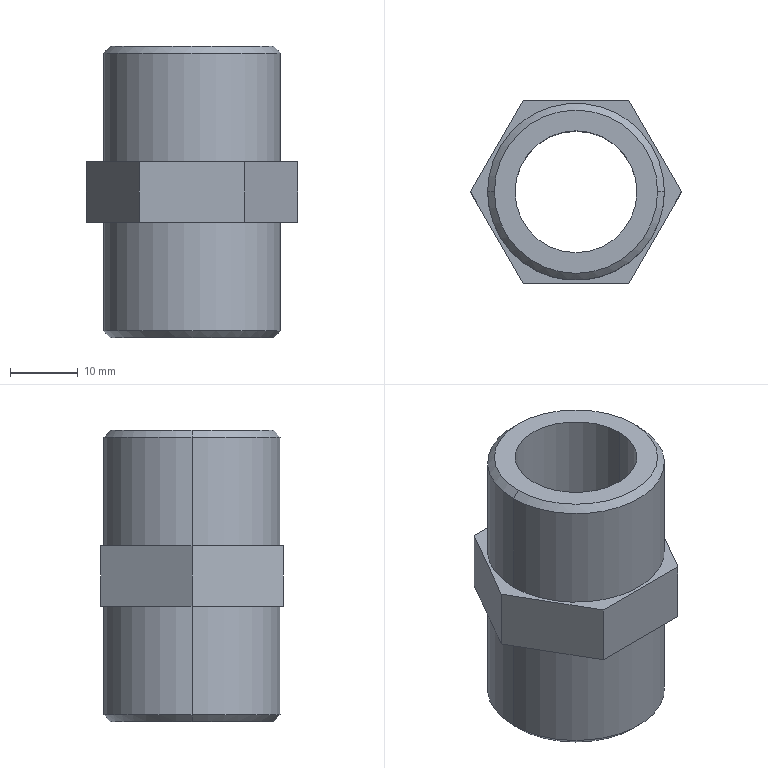Part | SolidWorks | features ICE 2, Chamfer 1, Extrusion 1, MirrorPattern 1 | 1 solid | 20 faces | box 31.177 x 27 x 43 mm | volume 12851 mm3 | plane 10 | cylinder 6 | cone 4 | commonest cylinder face diameters 26.1 x4 18 x2
STEP:
#1=CARTESIAN_POINT('',(12.05,0.,21.5));
#2=VERTEX_POINT('',#1);
#3=CARTESIAN_POINT('',(-12.05,0.,21.5));
#4=VERTEX_POINT('',#3);
#5=CARTESIAN_POINT('',(0.,0.,21.5));
#6=DIRECTION('',(0.,0.,1.));
#7=DIRECTION('',(1.,0.,0.));
#8=AXIS2_PLACEMENT_3D('',#5,#6,#7);
#9=CIRCLE('',#8,12.05);
#10=EDGE_CURVE('',#2,#4,#9,.T.);
#11=ORIENTED_EDGE('',*,*,#10,.F.);
#12=CARTESIAN_POINT('',(13.05,0.,20.5));
#13=VERTEX_POINT('',#12);
#14=CARTESIAN_POINT('',(13.05,0.,20.5));
#15=DIRECTION('',(0.7071,0.,-0.7071));
#16=VECTOR('',#15,1000.);
#17=LINE('',#14,#16);
#18=EDGE_CURVE('',#2,#13,#17,.T.);
#19=ORIENTED_EDGE('',*,*,#18,.T.);
#20=CARTESIAN_POINT('',(-13.05,0.,20.5));
#21=VERTEX_POINT('',#20);
#22=CARTESIAN_POINT('',(0.,0.,20.5));
#23=DIRECTION('',(0.,0.,-1.));
#24=DIRECTION('',(1.,0.,0.));
#25=AXIS2_PLACEMENT_3D('',#22,#23,#24);
#26=CIRCLE('',#25,13.05);
#27=EDGE_CURVE('',#21,#13,#26,.T.);
#28=ORIENTED_EDGE('',*,*,#27,.F.);
#29=CARTESIAN_POINT('',(-13.05,0.,20.5));
#30=DIRECTION('',(-0.7071,0.,-0.7071));
#31=VECTOR('',#30,1000.);
#32=LINE('',#29,#31);
#33=EDGE_CURVE('',#4,#21,#32,.T.);
#34=ORIENTED_EDGE('',*,*,#33,.F.);
#35=EDGE_LOOP('',(#11,#19,#28,#34));
#36=FACE_OUTER_BOUND('',#35,.T.);
#37=CARTESIAN_POINT('',(0.,0.,20.5));
#38=DIRECTION('',(0.,0.,-1.));
#39=DIRECTION('',(-1.,0.,0.));
#40=AXIS2_PLACEMENT_3D('',#37,#38,#39);
#41=CONICAL_SURFACE('',#40,13.05,0.7854);
#42=ADVANCED_FACE('',(#36),#41,.T.);
#43=CARTESIAN_POINT('',(-12.05,0.,-21.5));
#44=VERTEX_POINT('',#43);
#45=CARTESIAN_POINT('',(12.05,0.,-21.5));
#46=VERTEX_POINT('',#45);
#47=CARTESIAN_POINT('',(0.,0.,-21.5));
#48=DIRECTION('',(0.,0.,-1.));
#49=DIRECTION('',(-1.,0.,0.));
#50=AXIS2_PLACEMENT_3D('',#47,#48,#49);
#51=CIRCLE('',#50,12.05);
#52=EDGE_CURVE('',#44,#46,#51,.T.);
#53=ORIENTED_EDGE('',*,*,#52,.F.);
#54=CARTESIAN_POINT('',(-13.05,0.,-20.5));
#55=VERTEX_POINT('',#54);
#56=CARTESIAN_POINT('',(-12.05,0.,-21.5));
#57=DIRECTION('',(-0.7071,0.,0.7071));
#58=VECTOR('',#57,1000.);
#59=LINE('',#56,#58);
#60=EDGE_CURVE('',#44,#55,#59,.T.);
#61=ORIENTED_EDGE('',*,*,#60,.T.);
#62=CARTESIAN_POINT('',(13.05,0.,-20.5));
#63=VERTEX_POINT('',#62);
#64=CARTESIAN_POINT('',(0.,0.,-20.5));
#65=DIRECTION('',(0.,0.,1.));
#66=DIRECTION('',(-1.,0.,0.));
#67=AXIS2_PLACEMENT_3D('',#64,#65,#66);
#68=CIRCLE('',#67,13.05);
#69=EDGE_CURVE('',#63,#55,#68,.T.);
#70=ORIENTED_EDGE('',*,*,#69,.F.);
#71=CARTESIAN_POINT('',(12.05,0.,-21.5));
#72=DIRECTION('',(0.7071,0.,0.7071));
#73=VECTOR('',#72,1000.);
#74=LINE('',#71,#73);
#75=EDGE_CURVE('',#46,#63,#74,.T.);
#76=ORIENTED_EDGE('',*,*,#75,.F.);
#77=EDGE_LOOP('',(#53,#61,#70,#76));
#78=FACE_OUTER_BOUND('',#77,.T.);
#79=CARTESIAN_POINT('',(0.,0.,-21.5));
#80=DIRECTION('',(0.,0.,1.));
#81=DIRECTION('',(1.,0.,0.));
#82=AXIS2_PLACEMENT_3D('',#79,#80,#81);
#83=CONICAL_SURFACE('',#82,12.05,0.7854);
#84=ADVANCED_FACE('',(#78),#83,.T.);
#85=CARTESIAN_POINT('',(9.,0.,21.5));
#86=VERTEX_POINT('',#85);
#87=CARTESIAN_POINT('',(-9.,0.,21.5));
#88=VERTEX_POINT('',#87);
#89=CARTESIAN_POINT('',(0.,0.,21.5));
#90=DIRECTION('',(0.,0.,-1.));
#91=DIRECTION('',(1.,0.,0.));
#92=AXIS2_PLACEMENT_3D('',#89,#90,#91);
#93=CIRCLE('',#92,9.);
#94=EDGE_CURVE('',#86,#88,#93,.T.);
#95=ORIENTED_EDGE('',*,*,#94,.F.);
#96=CARTESIAN_POINT('',(9.,0.,-21.5));
#97=VERTEX_POINT('',#96);
#98=CARTESIAN_POINT('',(9.,0.,21.501));
#99=DIRECTION('',(0.,0.,-1.));
#100=VECTOR('',#99,1000.);
#101=LINE('',#98,#100);
#102=EDGE_CURVE('',#86,#97,#101,.T.);
#103=ORIENTED_EDGE('',*,*,#102,.T.);
#104=CARTESIAN_POINT('',(-9.,0.,-21.5));
#105=VERTEX_POINT('',#104);
#106=CARTESIAN_POINT('',(0.,0.,-21.5));
#107=DIRECTION('',(0.,0.,-1.));
#108=DIRECTION('',(-1.,0.,0.));
#109=AXIS2_PLACEMENT_3D('',#106,#107,#108);
#110=CIRCLE('',#109,9.);
#111=EDGE_CURVE('',#97,#105,#110,.T.);
#112=ORIENTED_EDGE('',*,*,#111,.T.);
#113=CARTESIAN_POINT('',(-9.,0.,21.501));
#114=DIRECTION('',(0.,0.,-1.));
#115=VECTOR('',#114,1000.);
#116=LINE('',#113,#115);
#117=EDGE_CURVE('',#88,#105,#116,.T.);
#118=ORIENTED_EDGE('',*,*,#117,.F.);
#119=EDGE_LOOP('',(#95,#103,#112,#118));
#120=FACE_OUTER_BOUND('',#119,.T.);
#121=CARTESIAN_POINT('',(0.,0.,21.501));
#122=DIRECTION('',(0.,0.,-1.));
#123=DIRECTION('',(-1.,0.,0.));
#124=AXIS2_PLACEMENT_3D('',#121,#122,#123);
#125=CYLINDRICAL_SURFACE('',#124,9.);
#126=ADVANCED_FACE('',(#120),#125,.F.);
#127=ORIENTED_EDGE('',*,*,#27,.T.);
#128=CARTESIAN_POINT('',(13.05,0.,4.5));
#129=VERTEX_POINT('',#128);
#130=CARTESIAN_POINT('',(13.05,0.,21.5));
#131=DIRECTION('',(0.,0.,-1.));
#132=VECTOR('',#131,1000.);
#133=LINE('',#130,#132);
#134=EDGE_CURVE('',#13,#129,#133,.T.);
#135=ORIENTED_EDGE('',*,*,#134,.T.);
#136=CARTESIAN_POINT('',(-13.05,0.,4.5));
#137=VERTEX_POINT('',#136);
#138=CARTESIAN_POINT('',(0.,0.,4.5));
#139=DIRECTION('',(0.,0.,-1.));
#140=DIRECTION('',(-1.,0.,0.));
#141=AXIS2_PLACEMENT_3D('',#138,#139,#140);
#142=CIRCLE('',#141,13.05);
#143=EDGE_CURVE('',#137,#129,#142,.T.);
#144=ORIENTED_EDGE('',*,*,#143,.F.);
#145=CARTESIAN_POINT('',(-13.05,0.,21.5));
#146=DIRECTION('',(0.,0.,-1.));
#147=VECTOR('',#146,1000.);
#148=LINE('',#145,#147);
#149=EDGE_CURVE('',#21,#137,#148,.T.);
#150=ORIENTED_EDGE('',*,*,#149,.F.);
#151=EDGE_LOOP('',(#127,#135,#144,#150));
#152=FACE_OUTER_BOUND('',#151,.T.);
#153=CARTESIAN_POINT('',(0.,0.,21.5));
#154=DIRECTION('',(0.,0.,-1.));
#155=DIRECTION('',(-1.,0.,0.));
#156=AXIS2_PLACEMENT_3D('',#153,#154,#155);
#157=CYLINDRICAL_SURFACE('',#156,13.05);
#158=ADVANCED_FACE('',(#152),#157,.T.);
#159=ORIENTED_EDGE('',*,*,#69,.T.);
#160=CARTESIAN_POINT('',(-13.05,0.,-4.5));
#161=VERTEX_POINT('',#160);
#162=CARTESIAN_POINT('',(-13.05,0.,-21.5));
#163=DIRECTION('',(0.,0.,1.));
#164=VECTOR('',#163,1000.);
#165=LINE('',#162,#164);
#166=EDGE_CURVE('',#55,#161,#165,.T.);
#167=ORIENTED_EDGE('',*,*,#166,.T.);
#168=CARTESIAN_POINT('',(13.05,0.,-4.5));
#169=VERTEX_POINT('',#168);
#170=CARTESIAN_POINT('',(0.,0.,-4.5));
#171=DIRECTION('',(0.,0.,-1.));
#172=DIRECTION('',(-1.,0.,0.));
#173=AXIS2_PLACEMENT_3D('',#170,#171,#172);
#174=CIRCLE('',#173,13.05);
#175=EDGE_CURVE('',#161,#169,#174,.T.);
#176=ORIENTED_EDGE('',*,*,#175,.T.);
#177=CARTESIAN_POINT('',(13.05,0.,-21.5));
#178=DIRECTION('',(0.,0.,1.));
#179=VECTOR('',#178,1000.);
#180=LINE('',#177,#179);
#181=EDGE_CURVE('',#63,#169,#180,.T.);
#182=ORIENTED_EDGE('',*,*,#181,.F.);
#183=EDGE_LOOP('',(#159,#167,#176,#182));
#184=FACE_OUTER_BOUND('',#183,.T.);
#185=CARTESIAN_POINT('',(0.,0.,-21.5));
#186=DIRECTION('',(0.,0.,1.));
#187=DIRECTION('',(1.,0.,0.));
#188=AXIS2_PLACEMENT_3D('',#185,#186,#187);
#189=CYLINDRICAL_SURFACE('',#188,13.05);
#190=ADVANCED_FACE('',(#184),#189,.T.);
#191=CARTESIAN_POINT('',(7.794,-13.5,-4.5));
#192=VERTEX_POINT('',#191);
#193=CARTESIAN_POINT('',(15.588,0.,-4.5));
#194=VERTEX_POINT('',#193);
#195=CARTESIAN_POINT('',(7.794,-13.5,-4.5));
#196=DIRECTION('',(0.5,0.866,0.));
#197=VECTOR('',#196,1000.);
#198=LINE('',#195,#197);
#199=EDGE_CURVE('',#192,#194,#198,.T.);
#200=ORIENTED_EDGE('',*,*,#199,.T.);
#201=CARTESIAN_POINT('',(15.588,0.,4.5));
#202=VERTEX_POINT('',#201);
#203=CARTESIAN_POINT('',(15.588,0.,4.5));
#204=DIRECTION('',(0.,0.,-1.));
#205=VECTOR('',#204,1000.);
#206=LINE('',#203,#205);
#207=EDGE_CURVE('',#202,#194,#206,.T.);
#208=ORIENTED_EDGE('',*,*,#207,.F.);
#209=CARTESIAN_POINT('',(7.794,-13.5,4.5));
#210=VERTEX_POINT('',#209);
#211=CARTESIAN_POINT('',(7.794,-13.5,4.5));
#212=DIRECTION('',(0.5,0.866,0.));
#213=VECTOR('',#212,1000.);
#214=LINE('',#211,#213);
#215=EDGE_CURVE('',#210,#202,#214,.T.);
#216=ORIENTED_EDGE('',*,*,#215,.F.);
#217=CARTESIAN_POINT('',(7.794,-13.5,4.5));
#218=DIRECTION('',(0.,0.,-1.));
#219=VECTOR('',#218,1000.);
#220=LINE('',#217,#219);
#221=EDGE_CURVE('',#210,#192,#220,.T.);
#222=ORIENTED_EDGE('',*,*,#221,.T.);
#223=EDGE_LOOP('',(#200,#208,#216,#222));
#224=FACE_OUTER_BOUND('',#223,.T.);
#225=CARTESIAN_POINT('',(7.794,-13.5,4.5));
#226=DIRECTION('',(-0.866,0.5,0.));
#227=DIRECTION('',(-0.5,-0.866,0.));
#228=AXIS2_PLACEMENT_3D('',#225,#226,#227);
#229=PLANE('',#228);
#230=ADVANCED_FACE('',(#224),#229,.F.);
#231=CARTESIAN_POINT('',(7.794,13.5,-4.5));
#232=VERTEX_POINT('',#231);
#233=CARTESIAN_POINT('',(15.588,0.,-4.5));
#234=DIRECTION('',(-0.5,0.866,0.));
#235=VECTOR('',#234,1000.);
#236=LINE('',#233,#235);
#237=EDGE_CURVE('',#194,#232,#236,.T.);
#238=ORIENTED_EDGE('',*,*,#237,.T.);
#239=CARTESIAN_POINT('',(7.794,13.5,4.5));
#240=VERTEX_POINT('',#239);
#241=CARTESIAN_POINT('',(7.794,13.5,4.5));
#242=DIRECTION('',(0.,0.,-1.));
#243=VECTOR('',#242,1000.);
#244=LINE('',#241,#243);
#245=EDGE_CURVE('',#240,#232,#244,.T.);
#246=ORIENTED_EDGE('',*,*,#245,.F.);
#247=CARTESIAN_POINT('',(15.588,0.,4.5));
#248=DIRECTION('',(-0.5,0.866,0.));
#249=VECTOR('',#248,1000.);
#250=LINE('',#247,#249);
#251=EDGE_CURVE('',#202,#240,#250,.T.);
#252=ORIENTED_EDGE('',*,*,#251,.F.);
#253=ORIENTED_EDGE('',*,*,#207,.T.);
#254=EDGE_LOOP('',(#238,#246,#252,#253));
#255=FACE_OUTER_BOUND('',#254,.T.);
#256=CARTESIAN_POINT('',(15.588,0.,4.5));
#257=DIRECTION('',(-0.866,-0.5,0.));
#258=DIRECTION('',(0.5,-0.866,0.));
#259=AXIS2_PLACEMENT_3D('',#256,#257,#258);
#260=PLANE('',#259);
#261=ADVANCED_FACE('',(#255),#260,.F.);
#262=CARTESIAN_POINT('',(-7.794,13.5,-4.5));
#263=VERTEX_POINT('',#262);
#264=CARTESIAN_POINT('',(7.794,13.5,-4.5));
#265=DIRECTION('',(-1.,0.,0.));
#266=VECTOR('',#265,1000.);
#267=LINE('',#264,#266);
#268=EDGE_CURVE('',#232,#263,#267,.T.);
#269=ORIENTED_EDGE('',*,*,#268,.T.);
#270=CARTESIAN_POINT('',(-7.794,13.5,4.5));
#271=VERTEX_POINT('',#270);
#272=CARTESIAN_POINT('',(-7.794,13.5,4.5));
#273=DIRECTION('',(0.,0.,-1.));
#274=VECTOR('',#273,1000.);
#275=LINE('',#272,#274);
#276=EDGE_CURVE('',#271,#263,#275,.T.);
#277=ORIENTED_EDGE('',*,*,#276,.F.);
#278=CARTESIAN_POINT('',(7.794,13.5,4.5));
#279=DIRECTION('',(-1.,0.,0.));
#280=VECTOR('',#279,1000.);
#281=LINE('',#278,#280);
#282=EDGE_CURVE('',#240,#271,#281,.T.);
#283=ORIENTED_EDGE('',*,*,#282,.F.);
#284=ORIENTED_EDGE('',*,*,#245,.T.);
#285=EDGE_LOOP('',(#269,#277,#283,#284));
#286=FACE_OUTER_BOUND('',#285,.T.);
#287=CARTESIAN_POINT('',(7.794,13.5,4.5));
#288=DIRECTION('',(0.,-1.,0.));
#289=DIRECTION('',(0.,0.,-1.));
#290=AXIS2_PLACEMENT_3D('',#287,#288,#289);
#291=PLANE('',#290);
#292=ADVANCED_FACE('',(#286),#291,.F.);
#293=CARTESIAN_POINT('',(-15.588,0.,-4.5));
#294=VERTEX_POINT('',#293);
#295=CARTESIAN_POINT('',(-7.794,13.5,-4.5));
#296=DIRECTION('',(-0.5,-0.866,0.));
#297=VECTOR('',#296,1000.);
#298=LINE('',#295,#297);
#299=EDGE_CURVE('',#263,#294,#298,.T.);
#300=ORIENTED_EDGE('',*,*,#299,.T.);
#301=CARTESIAN_POINT('',(-15.588,0.,4.5));
#302=VERTEX_POINT('',#301);
#303=CARTESIAN_POINT('',(-15.588,0.,4.5));
#304=DIRECTION('',(0.,0.,-1.));
#305=VECTOR('',#304,1000.);
#306=LINE('',#303,#305);
#307=EDGE_CURVE('',#302,#294,#306,.T.);
#308=ORIENTED_EDGE('',*,*,#307,.F.);
#309=CARTESIAN_POINT('',(-7.794,13.5,4.5));
#310=DIRECTION('',(-0.5,-0.866,0.));
#311=VECTOR('',#310,1000.);
#312=LINE('',#309,#311);
#313=EDGE_CURVE('',#271,#302,#312,.T.);
#314=ORIENTED_EDGE('',*,*,#313,.F.);
#315=ORIENTED_EDGE('',*,*,#276,.T.);
#316=EDGE_LOOP('',(#300,#308,#314,#315));
#317=FACE_OUTER_BOUND('',#316,.T.);
#318=CARTESIAN_POINT('',(-7.794,13.5,4.5));
#319=DIRECTION('',(0.866,-0.5,0.));
#320=DIRECTION('',(0.5,0.866,0.));
#321=AXIS2_PLACEMENT_3D('',#318,#319,#320);
#322=PLANE('',#321);
#323=ADVANCED_FACE('',(#317),#322,.F.);
#324=CARTESIAN_POINT('',(-7.794,-13.5,-4.5));
#325=VERTEX_POINT('',#324);
#326=CARTESIAN_POINT('',(-15.588,0.,-4.5));
#327=DIRECTION('',(0.5,-0.866,0.));
#328=VECTOR('',#327,1000.);
#329=LINE('',#326,#328);
#330=EDGE_CURVE('',#294,#325,#329,.T.);
#331=ORIENTED_EDGE('',*,*,#330,.T.);
#332=CARTESIAN_POINT('',(-7.794,-13.5,4.5));
#333=VERTEX_POINT('',#332);
#334=CARTESIAN_POINT('',(-7.794,-13.5,4.5));
#335=DIRECTION('',(0.,0.,-1.));
#336=VECTOR('',#335,1000.);
#337=LINE('',#334,#336);
#338=EDGE_CURVE('',#333,#325,#337,.T.);
#339=ORIENTED_EDGE('',*,*,#338,.F.);
#340=CARTESIAN_POINT('',(-15.588,0.,4.5));
#341=DIRECTION('',(0.5,-0.866,0.));
#342=VECTOR('',#341,1000.);
#343=LINE('',#340,#342);
#344=EDGE_CURVE('',#302,#333,#343,.T.);
#345=ORIENTED_EDGE('',*,*,#344,.F.);
#346=ORIENTED_EDGE('',*,*,#307,.T.);
#347=EDGE_LOOP('',(#331,#339,#345,#346));
#348=FACE_OUTER_BOUND('',#347,.T.);
#349=CARTESIAN_POINT('',(-15.588,0.,4.5));
#350=DIRECTION('',(0.866,0.5,0.));
#351=DIRECTION('',(-0.5,0.866,0.));
#352=AXIS2_PLACEMENT_3D('',#349,#350,#351);
#353=PLANE('',#352);
#354=ADVANCED_FACE('',(#348),#353,.F.);
#355=CARTESIAN_POINT('',(-7.794,-13.5,-4.5));
#356=DIRECTION('',(1.,0.,0.));
#357=VECTOR('',#356,1000.);
#358=LINE('',#355,#357);
#359=EDGE_CURVE('',#325,#192,#358,.T.);
#360=ORIENTED_EDGE('',*,*,#359,.T.);
#361=ORIENTED_EDGE('',*,*,#221,.F.);
#362=CARTESIAN_POINT('',(-7.794,-13.5,4.5));
#363=DIRECTION('',(1.,0.,0.));
#364=VECTOR('',#363,1000.);
#365=LINE('',#362,#364);
#366=EDGE_CURVE('',#333,#210,#365,.T.);
#367=ORIENTED_EDGE('',*,*,#366,.F.);
#368=ORIENTED_EDGE('',*,*,#338,.T.);
#369=EDGE_LOOP('',(#360,#361,#367,#368));
#370=FACE_OUTER_BOUND('',#369,.T.);
#371=CARTESIAN_POINT('',(-7.794,-13.5,4.5));
#372=DIRECTION('',(0.,1.,0.));
#373=DIRECTION('',(-1.,0.,0.));
#374=AXIS2_PLACEMENT_3D('',#371,#372,#373);
#375=PLANE('',#374);
#376=ADVANCED_FACE('',(#370),#375,.F.);
#377=ORIENTED_EDGE('',*,*,#143,.T.);
#378=CARTESIAN_POINT('',(0.,0.,4.5));
#379=DIRECTION('',(0.,0.,-1.));
#380=DIRECTION('',(-1.,0.,0.));
#381=AXIS2_PLACEMENT_3D('',#378,#379,#380);
#382=CIRCLE('',#381,13.05);
#383=EDGE_CURVE('',#129,#137,#382,.T.);
#384=ORIENTED_EDGE('',*,*,#383,.T.);
#385=EDGE_LOOP('',(#377,#384));
#386=FACE_BOUND('',#385,.T.);
#387=ORIENTED_EDGE('',*,*,#215,.T.);
#388=ORIENTED_EDGE('',*,*,#251,.T.);
#389=ORIENTED_EDGE('',*,*,#282,.T.);
#390=ORIENTED_EDGE('',*,*,#313,.T.);
#391=ORIENTED_EDGE('',*,*,#344,.T.);
#392=ORIENTED_EDGE('',*,*,#366,.T.);
#393=EDGE_LOOP('',(#387,#388,#389,#390,#391,#392));
#394=FACE_OUTER_BOUND('',#393,.T.);
#395=CARTESIAN_POINT('',(0.,0.,4.5));
#396=DIRECTION('',(0.,0.,1.));
#397=DIRECTION('',(1.,0.,0.));
#398=AXIS2_PLACEMENT_3D('',#395,#396,#397);
#399=PLANE('',#398);
#400=ADVANCED_FACE('',(#386,#394),#399,.T.);
#401=CARTESIAN_POINT('',(0.,0.,-4.5));
#402=DIRECTION('',(0.,0.,-1.));
#403=DIRECTION('',(-1.,0.,0.));
#404=AXIS2_PLACEMENT_3D('',#401,#402,#403);
#405=CIRCLE('',#404,13.05);
#406=EDGE_CURVE('',#169,#161,#405,.T.);
#407=ORIENTED_EDGE('',*,*,#406,.F.);
#408=ORIENTED_EDGE('',*,*,#175,.F.);
#409=EDGE_LOOP('',(#407,#408));
#410=FACE_BOUND('',#409,.T.);
#411=ORIENTED_EDGE('',*,*,#199,.F.);
#412=ORIENTED_EDGE('',*,*,#359,.F.);
#413=ORIENTED_EDGE('',*,*,#330,.F.);
#414=ORIENTED_EDGE('',*,*,#299,.F.);
#415=ORIENTED_EDGE('',*,*,#268,.F.);
#416=ORIENTED_EDGE('',*,*,#237,.F.);
#417=EDGE_LOOP('',(#411,#412,#413,#414,#415,#416));
#418=FACE_OUTER_BOUND('',#417,.T.);
#419=CARTESIAN_POINT('',(0.,0.,-4.5));
#420=DIRECTION('',(0.,0.,1.));
#421=DIRECTION('',(1.,0.,0.));
#422=AXIS2_PLACEMENT_3D('',#419,#420,#421);
#423=PLANE('',#422);
#424=ADVANCED_FACE('',(#410,#418),#423,.F.);
#425=ORIENTED_EDGE('',*,*,#166,.F.);
#426=CARTESIAN_POINT('',(0.,0.,-20.5));
#427=DIRECTION('',(0.,0.,1.));
#428=DIRECTION('',(-1.,0.,0.));
#429=AXIS2_PLACEMENT_3D('',#426,#427,#428);
#430=CIRCLE('',#429,13.05);
#431=EDGE_CURVE('',#55,#63,#430,.T.);
#432=ORIENTED_EDGE('',*,*,#431,.T.);
#433=ORIENTED_EDGE('',*,*,#181,.T.);
#434=ORIENTED_EDGE('',*,*,#406,.T.);
#435=EDGE_LOOP('',(#425,#432,#433,#434));
#436=FACE_OUTER_BOUND('',#435,.T.);
#437=CARTESIAN_POINT('',(0.,0.,-21.5));
#438=DIRECTION('',(0.,0.,1.));
#439=DIRECTION('',(1.,0.,0.));
#440=AXIS2_PLACEMENT_3D('',#437,#438,#439);
#441=CYLINDRICAL_SURFACE('',#440,13.05);
#442=ADVANCED_FACE('',(#436),#441,.T.);
#443=CARTESIAN_POINT('',(0.,0.,-21.5));
#444=DIRECTION('',(0.,0.,-1.));
#445=DIRECTION('',(-1.,0.,0.));
#446=AXIS2_PLACEMENT_3D('',#443,#444,#445);
#447=CIRCLE('',#446,12.05);
#448=EDGE_CURVE('',#46,#44,#447,.T.);
#449=ORIENTED_EDGE('',*,*,#448,.T.);
#450=ORIENTED_EDGE('',*,*,#52,.T.);
#451=EDGE_LOOP('',(#449,#450));
#452=FACE_OUTER_BOUND('',#451,.T.);
#453=CARTESIAN_POINT('',(0.,0.,-21.5));
#454=DIRECTION('',(0.,0.,-1.));
#455=DIRECTION('',(-1.,0.,0.));
#456=AXIS2_PLACEMENT_3D('',#453,#454,#455);
#457=CIRCLE('',#456,9.);
#458=EDGE_CURVE('',#105,#97,#457,.T.);
#459=ORIENTED_EDGE('',*,*,#458,.F.);
#460=ORIENTED_EDGE('',*,*,#111,.F.);
#461=EDGE_LOOP('',(#459,#460));
#462=FACE_BOUND('',#461,.T.);
#463=CARTESIAN_POINT('',(0.,0.,-21.5));
#464=DIRECTION('',(0.,0.,-1.));
#465=DIRECTION('',(-1.,0.,0.));
#466=AXIS2_PLACEMENT_3D('',#463,#464,#465);
#467=PLANE('',#466);
#468=ADVANCED_FACE('',(#452,#462),#467,.T.);
#469=ORIENTED_EDGE('',*,*,#134,.F.);
#470=CARTESIAN_POINT('',(0.,0.,20.5));
#471=DIRECTION('',(0.,0.,-1.));
#472=DIRECTION('',(1.,0.,0.));
#473=AXIS2_PLACEMENT_3D('',#470,#471,#472);
#474=CIRCLE('',#473,13.05);
#475=EDGE_CURVE('',#13,#21,#474,.T.);
#476=ORIENTED_EDGE('',*,*,#475,.T.);
#477=ORIENTED_EDGE('',*,*,#149,.T.);
#478=ORIENTED_EDGE('',*,*,#383,.F.);
#479=EDGE_LOOP('',(#469,#476,#477,#478));
#480=FACE_OUTER_BOUND('',#479,.T.);
#481=CARTESIAN_POINT('',(0.,0.,21.5));
#482=DIRECTION('',(0.,0.,-1.));
#483=DIRECTION('',(-1.,0.,0.));
#484=AXIS2_PLACEMENT_3D('',#481,#482,#483);
#485=CYLINDRICAL_SURFACE('',#484,13.05);
#486=ADVANCED_FACE('',(#480),#485,.T.);
#487=CARTESIAN_POINT('',(0.,0.,21.5));
#488=DIRECTION('',(0.,0.,1.));
#489=DIRECTION('',(1.,0.,0.));
#490=AXIS2_PLACEMENT_3D('',#487,#488,#489);
#491=CIRCLE('',#490,12.05);
#492=EDGE_CURVE('',#4,#2,#491,.T.);
#493=ORIENTED_EDGE('',*,*,#492,.T.);
#494=ORIENTED_EDGE('',*,*,#10,.T.);
#495=EDGE_LOOP('',(#493,#494));
#496=FACE_OUTER_BOUND('',#495,.T.);
#497=CARTESIAN_POINT('',(0.,0.,21.5));
#498=DIRECTION('',(0.,0.,-1.));
#499=DIRECTION('',(1.,0.,0.));
#500=AXIS2_PLACEMENT_3D('',#497,#498,#499);
#501=CIRCLE('',#500,9.);
#502=EDGE_CURVE('',#88,#86,#501,.T.);
#503=ORIENTED_EDGE('',*,*,#502,.T.);
#504=ORIENTED_EDGE('',*,*,#94,.T.);
#505=EDGE_LOOP('',(#503,#504));
#506=FACE_BOUND('',#505,.T.);
#507=CARTESIAN_POINT('',(0.,0.,21.5));
#508=DIRECTION('',(0.,0.,1.));
#509=DIRECTION('',(-1.,0.,0.));
#510=AXIS2_PLACEMENT_3D('',#507,#508,#509);
#511=PLANE('',#510);
#512=ADVANCED_FACE('',(#496,#506),#511,.T.);
#513=ORIENTED_EDGE('',*,*,#102,.F.);
#514=ORIENTED_EDGE('',*,*,#502,.F.);
#515=ORIENTED_EDGE('',*,*,#117,.T.);
#516=ORIENTED_EDGE('',*,*,#458,.T.);
#517=EDGE_LOOP('',(#513,#514,#515,#516));
#518=FACE_OUTER_BOUND('',#517,.T.);
#519=CARTESIAN_POINT('',(0.,0.,21.501));
#520=DIRECTION('',(0.,0.,-1.));
#521=DIRECTION('',(-1.,0.,0.));
#522=AXIS2_PLACEMENT_3D('',#519,#520,#521);
#523=CYLINDRICAL_SURFACE('',#522,9.);
#524=ADVANCED_FACE('',(#518),#523,.F.);
#525=ORIENTED_EDGE('',*,*,#60,.F.);
#526=ORIENTED_EDGE('',*,*,#448,.F.);
#527=ORIENTED_EDGE('',*,*,#75,.T.);
#528=ORIENTED_EDGE('',*,*,#431,.F.);
#529=EDGE_LOOP('',(#525,#526,#527,#528));
#530=FACE_OUTER_BOUND('',#529,.T.);
#531=CARTESIAN_POINT('',(0.,0.,-21.5));
#532=DIRECTION('',(0.,0.,1.));
#533=DIRECTION('',(1.,0.,0.));
#534=AXIS2_PLACEMENT_3D('',#531,#532,#533);
#535=CONICAL_SURFACE('',#534,12.05,0.7854);
#536=ADVANCED_FACE('',(#530),#535,.T.);
#537=ORIENTED_EDGE('',*,*,#18,.F.);
#538=ORIENTED_EDGE('',*,*,#492,.F.);
#539=ORIENTED_EDGE('',*,*,#33,.T.);
#540=ORIENTED_EDGE('',*,*,#475,.F.);
#541=EDGE_LOOP('',(#537,#538,#539,#540));
#542=FACE_OUTER_BOUND('',#541,.T.);
#543=CARTESIAN_POINT('',(0.,0.,20.5));
#544=DIRECTION('',(0.,0.,-1.));
#545=DIRECTION('',(-1.,0.,0.));
#546=AXIS2_PLACEMENT_3D('',#543,#544,#545);
#547=CONICAL_SURFACE('',#546,13.05,0.7854);
#548=ADVANCED_FACE('',(#542),#547,.T.);
#549=CLOSED_SHELL('',(#42,#84,#126,#158,#190,#230,#261,#292,#323,#354,#376,#400,#424,#442,#468,#486,#512,#524,#536,#548));
#550=MANIFOLD_SOLID_BREP('',#549);
#551=CARTESIAN_POINT('',(0.,0.,0.));
#552=DIRECTION('',(0.,0.,1.));
#553=DIRECTION('',(1.,0.,0.));
#554=AXIS2_PLACEMENT_3D('',#551,#552,#553);
#555=(LENGTH_UNIT()NAMED_UNIT(*)SI_UNIT(.MILLI.,.METRE.));
#556=UNCERTAINTY_MEASURE_WITH_UNIT(LENGTH_MEASURE(0.00001),#555,'','');
#557=(NAMED_UNIT(*)PLANE_ANGLE_UNIT()SI_UNIT($,.RADIAN.));
#558=(NAMED_UNIT(*)SI_UNIT($,.STERADIAN.)SOLID_ANGLE_UNIT());
#559=(GEOMETRIC_REPRESENTATION_CONTEXT(3)GLOBAL_UNCERTAINTY_ASSIGNED_CONTEXT((#556))GLOBAL_UNIT_ASSIGNED_CONTEXT((#555,#557,#558))REPRESENTATION_CONTEXT('',''));
#560=ADVANCED_BREP_SHAPE_REPRESENTATION('',(#550,#554),#559);